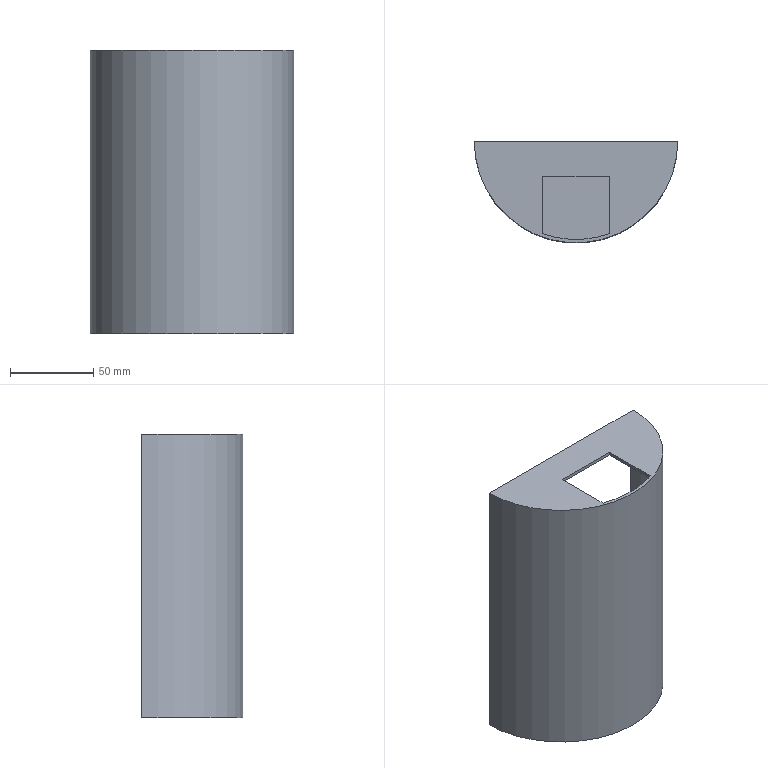Part | NX | 1 solid | 10 faces | box 122 x 61 x 170 mm | volume 83012 mm3 | plane 8 | cylinder 2 | commonest cylinder face diameters 118 x1 122 x1
STEP:
#1=CARTESIAN_POINT('',(61.,0.,0.));
#2=VERTEX_POINT('',#1);
#3=CARTESIAN_POINT('',(-61.,0.,0.));
#4=VERTEX_POINT('',#3);
#5=CARTESIAN_POINT('',(-61.,0.,0.));
#6=DIRECTION('',(-1.,0.,0.));
#7=VECTOR('',#6,1.);
#8=LINE('',#5,#7);
#9=EDGE_CURVE('',#2,#4,#8,.T.);
#10=ORIENTED_EDGE('',*,*,#9,.F.);
#11=CARTESIAN_POINT('',(61.,0.,-170.));
#12=VERTEX_POINT('',#11);
#13=CARTESIAN_POINT('',(61.,0.,-170.));
#14=DIRECTION('',(0.,0.,1.));
#15=VECTOR('',#14,1.);
#16=LINE('',#13,#15);
#17=EDGE_CURVE('',#12,#2,#16,.T.);
#18=ORIENTED_EDGE('',*,*,#17,.F.);
#19=CARTESIAN_POINT('',(-61.,0.,-170.));
#20=VERTEX_POINT('',#19);
#21=CARTESIAN_POINT('',(-61.,0.,-170.));
#22=DIRECTION('',(-1.,0.,0.));
#23=VECTOR('',#22,1.);
#24=LINE('',#21,#23);
#25=EDGE_CURVE('',#12,#20,#24,.T.);
#26=ORIENTED_EDGE('',*,*,#25,.T.);
#27=CARTESIAN_POINT('',(-61.,0.,-170.));
#28=DIRECTION('',(0.,0.,1.));
#29=VECTOR('',#28,1.);
#30=LINE('',#27,#29);
#31=EDGE_CURVE('',#20,#4,#30,.T.);
#32=ORIENTED_EDGE('',*,*,#31,.T.);
#33=EDGE_LOOP('',(#10,#18,#26,#32));
#34=FACE_BOUND('',#33,.T.);
#35=CARTESIAN_POINT('',(59.,0.,-2.));
#36=VERTEX_POINT('',#35);
#37=CARTESIAN_POINT('',(59.,0.,-168.));
#38=VERTEX_POINT('',#37);
#39=CARTESIAN_POINT('',(59.,0.,-168.));
#40=DIRECTION('',(0.,0.,-1.));
#41=VECTOR('',#40,1.);
#42=LINE('',#39,#41);
#43=EDGE_CURVE('',#36,#38,#42,.T.);
#44=ORIENTED_EDGE('',*,*,#43,.F.);
#45=CARTESIAN_POINT('',(-59.,0.,-2.));
#46=VERTEX_POINT('',#45);
#47=CARTESIAN_POINT('',(0.,0.,-2.));
#48=DIRECTION('',(-1.,0.,0.));
#49=VECTOR('',#48,1.);
#50=LINE('',#47,#49);
#51=EDGE_CURVE('',#36,#46,#50,.T.);
#52=ORIENTED_EDGE('',*,*,#51,.T.);
#53=CARTESIAN_POINT('',(-59.,0.,-168.));
#54=VERTEX_POINT('',#53);
#55=CARTESIAN_POINT('',(-59.,0.,-168.));
#56=DIRECTION('',(0.,0.,-1.));
#57=VECTOR('',#56,1.);
#58=LINE('',#55,#57);
#59=EDGE_CURVE('',#46,#54,#58,.T.);
#60=ORIENTED_EDGE('',*,*,#59,.T.);
#61=CARTESIAN_POINT('',(0.,0.,-168.));
#62=DIRECTION('',(-1.,0.,0.));
#63=VECTOR('',#62,1.);
#64=LINE('',#61,#63);
#65=EDGE_CURVE('',#38,#54,#64,.T.);
#66=ORIENTED_EDGE('',*,*,#65,.F.);
#67=EDGE_LOOP('',(#44,#52,#60,#66));
#68=FACE_BOUND('',#67,.T.);
#69=CARTESIAN_POINT('',(-61.,0.,-170.));
#70=DIRECTION('',(0.,1.,0.));
#71=DIRECTION('',(0.,0.,1.));
#72=AXIS2_PLACEMENT_3D('',#69,#70,#71);
#73=PLANE('',#72);
#74=ADVANCED_FACE('',(#34,#68),#73,.T.);
#75=CARTESIAN_POINT('',(0.,0.,0.));
#76=DIRECTION('',(0.,0.,1.));
#77=DIRECTION('',(1.,0.,0.));
#78=AXIS2_PLACEMENT_3D('',#75,#76,#77);
#79=CIRCLE('',#78,61.);
#80=EDGE_CURVE('',#4,#2,#79,.T.);
#81=ORIENTED_EDGE('',*,*,#80,.F.);
#82=ORIENTED_EDGE('',*,*,#31,.F.);
#83=CARTESIAN_POINT('',(0.,0.,-170.));
#84=DIRECTION('',(0.,0.,1.));
#85=DIRECTION('',(1.,0.,0.));
#86=AXIS2_PLACEMENT_3D('',#83,#84,#85);
#87=CIRCLE('',#86,61.);
#88=EDGE_CURVE('',#20,#12,#87,.T.);
#89=ORIENTED_EDGE('',*,*,#88,.T.);
#90=ORIENTED_EDGE('',*,*,#17,.T.);
#91=EDGE_LOOP('',(#81,#82,#89,#90));
#92=FACE_OUTER_BOUND('',#91,.T.);
#93=CARTESIAN_POINT('',(0.,0.,-170.));
#94=DIRECTION('',(0.,0.,1.));
#95=DIRECTION('',(1.,0.,0.));
#96=AXIS2_PLACEMENT_3D('',#93,#94,#95);
#97=CYLINDRICAL_SURFACE('',#96,61.);
#98=ADVANCED_FACE('',(#92),#97,.T.);
#99=ORIENTED_EDGE('',*,*,#88,.F.);
#100=ORIENTED_EDGE('',*,*,#25,.F.);
#101=EDGE_LOOP('',(#99,#100));
#102=FACE_OUTER_BOUND('',#101,.T.);
#103=CARTESIAN_POINT('',(0.,0.,-170.));
#104=DIRECTION('',(0.,0.,1.));
#105=DIRECTION('',(1.,0.,0.));
#106=AXIS2_PLACEMENT_3D('',#103,#104,#105);
#107=PLANE('',#106);
#108=ADVANCED_FACE('',(#102),#107,.F.);
#109=CARTESIAN_POINT('',(20.,-55.507,0.));
#110=VERTEX_POINT('',#109);
#111=CARTESIAN_POINT('',(20.,-21.,0.));
#112=VERTEX_POINT('',#111);
#113=CARTESIAN_POINT('',(20.,-21.,0.));
#114=DIRECTION('',(0.,1.,0.));
#115=VECTOR('',#114,1.);
#116=LINE('',#113,#115);
#117=EDGE_CURVE('',#110,#112,#116,.T.);
#118=ORIENTED_EDGE('',*,*,#117,.F.);
#119=CARTESIAN_POINT('',(-20.,-55.507,0.));
#120=VERTEX_POINT('',#119);
#121=CARTESIAN_POINT('',(0.,0.,0.));
#122=DIRECTION('',(0.,0.,1.));
#123=DIRECTION('',(1.,0.,0.));
#124=AXIS2_PLACEMENT_3D('',#121,#122,#123);
#125=CIRCLE('',#124,59.);
#126=EDGE_CURVE('',#120,#110,#125,.T.);
#127=ORIENTED_EDGE('',*,*,#126,.F.);
#128=CARTESIAN_POINT('',(-20.,-21.,0.));
#129=VERTEX_POINT('',#128);
#130=CARTESIAN_POINT('',(-20.,-21.,0.));
#131=DIRECTION('',(0.,-1.,0.));
#132=VECTOR('',#131,1.);
#133=LINE('',#130,#132);
#134=EDGE_CURVE('',#129,#120,#133,.T.);
#135=ORIENTED_EDGE('',*,*,#134,.F.);
#136=CARTESIAN_POINT('',(-20.,-21.,0.));
#137=DIRECTION('',(-1.,0.,0.));
#138=VECTOR('',#137,1.);
#139=LINE('',#136,#138);
#140=EDGE_CURVE('',#112,#129,#139,.T.);
#141=ORIENTED_EDGE('',*,*,#140,.F.);
#142=EDGE_LOOP('',(#118,#127,#135,#141));
#143=FACE_BOUND('',#142,.T.);
#144=ORIENTED_EDGE('',*,*,#80,.T.);
#145=ORIENTED_EDGE('',*,*,#9,.T.);
#146=EDGE_LOOP('',(#144,#145));
#147=FACE_BOUND('',#146,.T.);
#148=CARTESIAN_POINT('',(0.,0.,0.));
#149=DIRECTION('',(0.,0.,1.));
#150=DIRECTION('',(1.,0.,0.));
#151=AXIS2_PLACEMENT_3D('',#148,#149,#150);
#152=PLANE('',#151);
#153=ADVANCED_FACE('',(#143,#147),#152,.T.);
#154=CARTESIAN_POINT('',(-20.,-55.507,-2.));
#155=VERTEX_POINT('',#154);
#156=CARTESIAN_POINT('',(0.,0.,-2.));
#157=DIRECTION('',(0.,0.,1.));
#158=DIRECTION('',(1.,0.,0.));
#159=AXIS2_PLACEMENT_3D('',#156,#157,#158);
#160=CIRCLE('',#159,59.);
#161=EDGE_CURVE('',#46,#155,#160,.T.);
#162=ORIENTED_EDGE('',*,*,#161,.T.);
#163=CARTESIAN_POINT('',(-20.,-55.507,-2.));
#164=DIRECTION('',(0.,0.,1.));
#165=VECTOR('',#164,1.);
#166=LINE('',#163,#165);
#167=EDGE_CURVE('',#155,#120,#166,.T.);
#168=ORIENTED_EDGE('',*,*,#167,.T.);
#169=ORIENTED_EDGE('',*,*,#126,.T.);
#170=CARTESIAN_POINT('',(20.,-55.507,-2.));
#171=VERTEX_POINT('',#170);
#172=CARTESIAN_POINT('',(20.,-55.507,-2.));
#173=DIRECTION('',(0.,0.,1.));
#174=VECTOR('',#173,1.);
#175=LINE('',#172,#174);
#176=EDGE_CURVE('',#171,#110,#175,.T.);
#177=ORIENTED_EDGE('',*,*,#176,.F.);
#178=CARTESIAN_POINT('',(0.,0.,-2.));
#179=DIRECTION('',(0.,0.,1.));
#180=DIRECTION('',(1.,0.,0.));
#181=AXIS2_PLACEMENT_3D('',#178,#179,#180);
#182=CIRCLE('',#181,59.);
#183=EDGE_CURVE('',#171,#36,#182,.T.);
#184=ORIENTED_EDGE('',*,*,#183,.T.);
#185=ORIENTED_EDGE('',*,*,#43,.T.);
#186=CARTESIAN_POINT('',(0.,0.,-168.));
#187=DIRECTION('',(0.,0.,1.));
#188=DIRECTION('',(1.,0.,0.));
#189=AXIS2_PLACEMENT_3D('',#186,#187,#188);
#190=CIRCLE('',#189,59.);
#191=EDGE_CURVE('',#54,#38,#190,.T.);
#192=ORIENTED_EDGE('',*,*,#191,.F.);
#193=ORIENTED_EDGE('',*,*,#59,.F.);
#194=EDGE_LOOP('',(#162,#168,#169,#177,#184,#185,#192,#193));
#195=FACE_OUTER_BOUND('',#194,.T.);
#196=CARTESIAN_POINT('',(0.,0.,-170.));
#197=DIRECTION('',(0.,0.,1.));
#198=DIRECTION('',(1.,0.,0.));
#199=AXIS2_PLACEMENT_3D('',#196,#197,#198);
#200=CYLINDRICAL_SURFACE('',#199,59.);
#201=ADVANCED_FACE('',(#195),#200,.F.);
#202=ORIENTED_EDGE('',*,*,#191,.T.);
#203=ORIENTED_EDGE('',*,*,#65,.T.);
#204=EDGE_LOOP('',(#202,#203));
#205=FACE_OUTER_BOUND('',#204,.T.);
#206=CARTESIAN_POINT('',(0.,0.,-168.));
#207=DIRECTION('',(0.,0.,1.));
#208=DIRECTION('',(1.,0.,0.));
#209=AXIS2_PLACEMENT_3D('',#206,#207,#208);
#210=PLANE('',#209);
#211=ADVANCED_FACE('',(#205),#210,.T.);
#212=ORIENTED_EDGE('',*,*,#183,.F.);
#213=CARTESIAN_POINT('',(20.,-21.,-2.));
#214=VERTEX_POINT('',#213);
#215=CARTESIAN_POINT('',(20.,-21.,-2.));
#216=DIRECTION('',(0.,1.,0.));
#217=VECTOR('',#216,1.);
#218=LINE('',#215,#217);
#219=EDGE_CURVE('',#171,#214,#218,.T.);
#220=ORIENTED_EDGE('',*,*,#219,.T.);
#221=CARTESIAN_POINT('',(-20.,-21.,-2.));
#222=VERTEX_POINT('',#221);
#223=CARTESIAN_POINT('',(-20.,-21.,-2.));
#224=DIRECTION('',(-1.,0.,0.));
#225=VECTOR('',#224,1.);
#226=LINE('',#223,#225);
#227=EDGE_CURVE('',#214,#222,#226,.T.);
#228=ORIENTED_EDGE('',*,*,#227,.T.);
#229=CARTESIAN_POINT('',(-20.,-21.,-2.));
#230=DIRECTION('',(0.,-1.,0.));
#231=VECTOR('',#230,1.);
#232=LINE('',#229,#231);
#233=EDGE_CURVE('',#222,#155,#232,.T.);
#234=ORIENTED_EDGE('',*,*,#233,.T.);
#235=ORIENTED_EDGE('',*,*,#161,.F.);
#236=ORIENTED_EDGE('',*,*,#51,.F.);
#237=EDGE_LOOP('',(#212,#220,#228,#234,#235,#236));
#238=FACE_OUTER_BOUND('',#237,.T.);
#239=CARTESIAN_POINT('',(0.,0.,-2.));
#240=DIRECTION('',(0.,0.,1.));
#241=DIRECTION('',(1.,0.,0.));
#242=AXIS2_PLACEMENT_3D('',#239,#240,#241);
#243=PLANE('',#242);
#244=ADVANCED_FACE('',(#238),#243,.F.);
#245=ORIENTED_EDGE('',*,*,#117,.T.);
#246=CARTESIAN_POINT('',(20.,-21.,-2.));
#247=DIRECTION('',(0.,0.,1.));
#248=VECTOR('',#247,1.);
#249=LINE('',#246,#248);
#250=EDGE_CURVE('',#214,#112,#249,.T.);
#251=ORIENTED_EDGE('',*,*,#250,.F.);
#252=ORIENTED_EDGE('',*,*,#219,.F.);
#253=ORIENTED_EDGE('',*,*,#176,.T.);
#254=EDGE_LOOP('',(#245,#251,#252,#253));
#255=FACE_OUTER_BOUND('',#254,.T.);
#256=CARTESIAN_POINT('',(20.,-21.,-2.));
#257=DIRECTION('',(1.,0.,0.));
#258=DIRECTION('',(0.,1.,0.));
#259=AXIS2_PLACEMENT_3D('',#256,#257,#258);
#260=PLANE('',#259);
#261=ADVANCED_FACE('',(#255),#260,.F.);
#262=ORIENTED_EDGE('',*,*,#134,.T.);
#263=ORIENTED_EDGE('',*,*,#167,.F.);
#264=ORIENTED_EDGE('',*,*,#233,.F.);
#265=CARTESIAN_POINT('',(-20.,-21.,-2.));
#266=DIRECTION('',(0.,0.,1.));
#267=VECTOR('',#266,1.);
#268=LINE('',#265,#267);
#269=EDGE_CURVE('',#222,#129,#268,.T.);
#270=ORIENTED_EDGE('',*,*,#269,.T.);
#271=EDGE_LOOP('',(#262,#263,#264,#270));
#272=FACE_OUTER_BOUND('',#271,.T.);
#273=CARTESIAN_POINT('',(-20.,-21.,-2.));
#274=DIRECTION('',(-1.,0.,0.));
#275=DIRECTION('',(0.,-1.,0.));
#276=AXIS2_PLACEMENT_3D('',#273,#274,#275);
#277=PLANE('',#276);
#278=ADVANCED_FACE('',(#272),#277,.F.);
#279=ORIENTED_EDGE('',*,*,#140,.T.);
#280=ORIENTED_EDGE('',*,*,#269,.F.);
#281=ORIENTED_EDGE('',*,*,#227,.F.);
#282=ORIENTED_EDGE('',*,*,#250,.T.);
#283=EDGE_LOOP('',(#279,#280,#281,#282));
#284=FACE_OUTER_BOUND('',#283,.T.);
#285=CARTESIAN_POINT('',(-20.,-21.,-2.));
#286=DIRECTION('',(0.,1.,0.));
#287=DIRECTION('',(-1.,0.,0.));
#288=AXIS2_PLACEMENT_3D('',#285,#286,#287);
#289=PLANE('',#288);
#290=ADVANCED_FACE('',(#284),#289,.F.);
#291=CLOSED_SHELL('',(#74,#98,#108,#153,#201,#211,#244,#261,#278,#290));
#292=MANIFOLD_SOLID_BREP('',#291);
#293=(LENGTH_UNIT()NAMED_UNIT(*)SI_UNIT(.MILLI.,.METRE.));
#294=UNCERTAINTY_MEASURE_WITH_UNIT(LENGTH_MEASURE(0.00002),#293,'','');
#295=(NAMED_UNIT(*)PLANE_ANGLE_UNIT()SI_UNIT($,.RADIAN.));
#296=PLANE_ANGLE_MEASURE_WITH_UNIT(PLANE_ANGLE_MEASURE(0.01745),#295);
#297=DIMENSIONAL_EXPONENTS(0.,0.,0.,0.,0.,0.,0.);
#298=(CONVERSION_BASED_UNIT('DEGREE',#296)NAMED_UNIT(#297)PLANE_ANGLE_UNIT());
#299=(NAMED_UNIT(*)SI_UNIT($,.STERADIAN.)SOLID_ANGLE_UNIT());
#300=(GEOMETRIC_REPRESENTATION_CONTEXT(3)GLOBAL_UNCERTAINTY_ASSIGNED_CONTEXT((#294))GLOBAL_UNIT_ASSIGNED_CONTEXT((#293,#298,#299))REPRESENTATION_CONTEXT('',''));
#301=ADVANCED_BREP_SHAPE_REPRESENTATION('',(#292),#300);